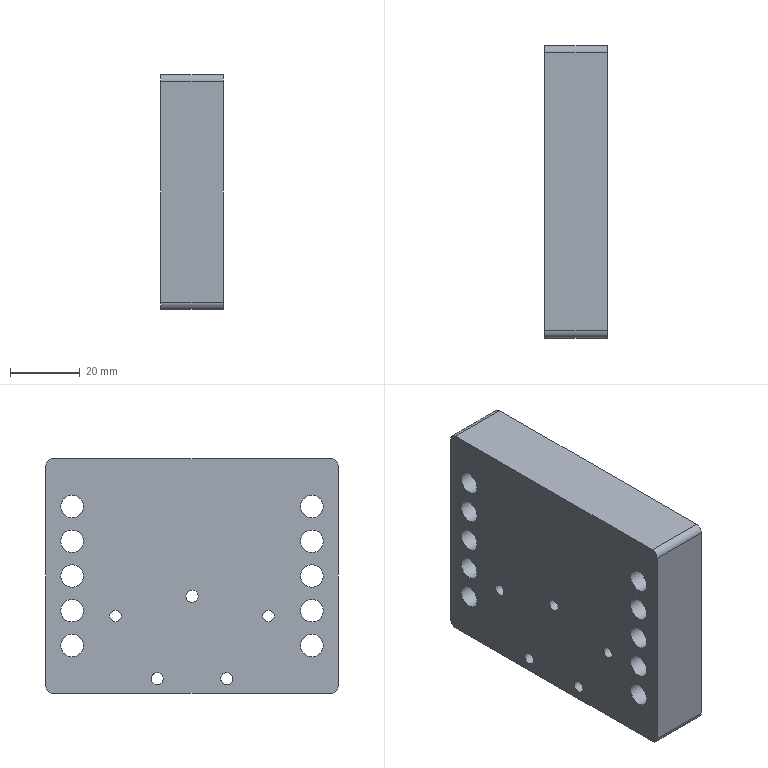Part | NX | 1 solid | 31 faces | box 18 x 84 x 67.5 mm | volume 94862 mm3 | cylinder 22 | plane 9 | commonest cylinder face diameters 6.5 x10 4 x4 3.5 x3 6 x3 3.3 x2
STEP:
#1=CARTESIAN_POINT('',(-224.,-62.153,788.95));
#2=VERTEX_POINT('',#1);
#3=CARTESIAN_POINT('',(-224.,-65.403,788.95));
#4=DIRECTION('',(1.,0.,0.));
#5=DIRECTION('',(0.,1.,0.));
#6=AXIS2_PLACEMENT_3D('',#3,#4,#5);
#7=CIRCLE('',#6,3.25);
#8=EDGE_CURVE('',#2,#2,#7,.T.);
#9=ORIENTED_EDGE('',*,*,#8,.T.);
#10=EDGE_LOOP('',(#9));
#11=FACE_BOUND('',#10,.T.);
#12=CARTESIAN_POINT('',(-224.,-62.153,778.95));
#13=VERTEX_POINT('',#12);
#14=CARTESIAN_POINT('',(-224.,-65.403,778.95));
#15=DIRECTION('',(1.,0.,0.));
#16=DIRECTION('',(0.,1.,0.));
#17=AXIS2_PLACEMENT_3D('',#14,#15,#16);
#18=CIRCLE('',#17,3.25);
#19=EDGE_CURVE('',#13,#13,#18,.T.);
#20=ORIENTED_EDGE('',*,*,#19,.T.);
#21=EDGE_LOOP('',(#20));
#22=FACE_BOUND('',#21,.T.);
#23=CARTESIAN_POINT('',(-224.,-62.153,748.95));
#24=VERTEX_POINT('',#23);
#25=CARTESIAN_POINT('',(-224.,-65.403,748.95));
#26=DIRECTION('',(1.,0.,0.));
#27=DIRECTION('',(0.,1.,0.));
#28=AXIS2_PLACEMENT_3D('',#25,#26,#27);
#29=CIRCLE('',#28,3.25);
#30=EDGE_CURVE('',#24,#24,#29,.T.);
#31=ORIENTED_EDGE('',*,*,#30,.T.);
#32=EDGE_LOOP('',(#31));
#33=FACE_BOUND('',#32,.T.);
#34=CARTESIAN_POINT('',(-224.,-62.153,758.95));
#35=VERTEX_POINT('',#34);
#36=CARTESIAN_POINT('',(-224.,-65.403,758.95));
#37=DIRECTION('',(1.,0.,0.));
#38=DIRECTION('',(0.,1.,0.));
#39=AXIS2_PLACEMENT_3D('',#36,#37,#38);
#40=CIRCLE('',#39,3.25);
#41=EDGE_CURVE('',#35,#35,#40,.T.);
#42=ORIENTED_EDGE('',*,*,#41,.T.);
#43=EDGE_LOOP('',(#42));
#44=FACE_BOUND('',#43,.T.);
#45=CARTESIAN_POINT('',(-224.,-62.153,768.95));
#46=VERTEX_POINT('',#45);
#47=CARTESIAN_POINT('',(-224.,-65.403,768.95));
#48=DIRECTION('',(1.,0.,0.));
#49=DIRECTION('',(0.,1.,0.));
#50=AXIS2_PLACEMENT_3D('',#47,#48,#49);
#51=CIRCLE('',#50,3.25);
#52=EDGE_CURVE('',#46,#46,#51,.T.);
#53=ORIENTED_EDGE('',*,*,#52,.T.);
#54=EDGE_LOOP('',(#53));
#55=FACE_BOUND('',#54,.T.);
#56=CARTESIAN_POINT('',(-224.,-131.153,748.95));
#57=VERTEX_POINT('',#56);
#58=CARTESIAN_POINT('',(-224.,-134.403,748.95));
#59=DIRECTION('',(1.,0.,0.));
#60=DIRECTION('',(0.,1.,0.));
#61=AXIS2_PLACEMENT_3D('',#58,#59,#60);
#62=CIRCLE('',#61,3.25);
#63=EDGE_CURVE('',#57,#57,#62,.T.);
#64=ORIENTED_EDGE('',*,*,#63,.T.);
#65=EDGE_LOOP('',(#64));
#66=FACE_BOUND('',#65,.T.);
#67=CARTESIAN_POINT('',(-224.,-131.153,758.95));
#68=VERTEX_POINT('',#67);
#69=CARTESIAN_POINT('',(-224.,-134.403,758.95));
#70=DIRECTION('',(1.,0.,0.));
#71=DIRECTION('',(0.,1.,0.));
#72=AXIS2_PLACEMENT_3D('',#69,#70,#71);
#73=CIRCLE('',#72,3.25);
#74=EDGE_CURVE('',#68,#68,#73,.T.);
#75=ORIENTED_EDGE('',*,*,#74,.T.);
#76=EDGE_LOOP('',(#75));
#77=FACE_BOUND('',#76,.T.);
#78=CARTESIAN_POINT('',(-224.,-131.153,788.95));
#79=VERTEX_POINT('',#78);
#80=CARTESIAN_POINT('',(-224.,-134.403,788.95));
#81=DIRECTION('',(1.,0.,0.));
#82=DIRECTION('',(0.,1.,0.));
#83=AXIS2_PLACEMENT_3D('',#80,#81,#82);
#84=CIRCLE('',#83,3.25);
#85=EDGE_CURVE('',#79,#79,#84,.T.);
#86=ORIENTED_EDGE('',*,*,#85,.T.);
#87=EDGE_LOOP('',(#86));
#88=FACE_BOUND('',#87,.T.);
#89=CARTESIAN_POINT('',(-224.,-131.153,778.95));
#90=VERTEX_POINT('',#89);
#91=CARTESIAN_POINT('',(-224.,-134.403,778.95));
#92=DIRECTION('',(1.,0.,0.));
#93=DIRECTION('',(0.,1.,0.));
#94=AXIS2_PLACEMENT_3D('',#91,#92,#93);
#95=CIRCLE('',#94,3.25);
#96=EDGE_CURVE('',#90,#90,#95,.T.);
#97=ORIENTED_EDGE('',*,*,#96,.T.);
#98=EDGE_LOOP('',(#97));
#99=FACE_BOUND('',#98,.T.);
#100=CARTESIAN_POINT('',(-224.,-131.153,768.95));
#101=VERTEX_POINT('',#100);
#102=CARTESIAN_POINT('',(-224.,-134.403,768.95));
#103=DIRECTION('',(1.,0.,0.));
#104=DIRECTION('',(0.,1.,0.));
#105=AXIS2_PLACEMENT_3D('',#102,#103,#104);
#106=CIRCLE('',#105,3.25);
#107=EDGE_CURVE('',#101,#101,#106,.T.);
#108=ORIENTED_EDGE('',*,*,#107,.T.);
#109=EDGE_LOOP('',(#108));
#110=FACE_BOUND('',#109,.T.);
#111=CARTESIAN_POINT('',(-224.,-120.253,757.45));
#112=VERTEX_POINT('',#111);
#113=CARTESIAN_POINT('',(-224.,-121.903,757.45));
#114=DIRECTION('',(-1.,0.,0.));
#115=DIRECTION('',(0.,1.,0.));
#116=AXIS2_PLACEMENT_3D('',#113,#114,#115);
#117=CIRCLE('',#116,1.65);
#118=EDGE_CURVE('',#112,#112,#117,.T.);
#119=ORIENTED_EDGE('',*,*,#118,.F.);
#120=EDGE_LOOP('',(#119));
#121=FACE_BOUND('',#120,.T.);
#122=CARTESIAN_POINT('',(-224.,-76.253,757.45));
#123=VERTEX_POINT('',#122);
#124=CARTESIAN_POINT('',(-224.,-77.903,757.45));
#125=DIRECTION('',(-1.,0.,0.));
#126=DIRECTION('',(0.,1.,0.));
#127=AXIS2_PLACEMENT_3D('',#124,#125,#126);
#128=CIRCLE('',#127,1.65);
#129=EDGE_CURVE('',#123,#123,#128,.T.);
#130=ORIENTED_EDGE('',*,*,#129,.F.);
#131=EDGE_LOOP('',(#130));
#132=FACE_BOUND('',#131,.T.);
#133=CARTESIAN_POINT('',(-224.,-108.153,739.4));
#134=VERTEX_POINT('',#133);
#135=CARTESIAN_POINT('',(-224.,-109.903,739.4));
#136=DIRECTION('',(1.,0.,0.));
#137=DIRECTION('',(0.,1.,0.));
#138=AXIS2_PLACEMENT_3D('',#135,#136,#137);
#139=CIRCLE('',#138,1.75);
#140=EDGE_CURVE('',#134,#134,#139,.T.);
#141=ORIENTED_EDGE('',*,*,#140,.T.);
#142=EDGE_LOOP('',(#141));
#143=FACE_BOUND('',#142,.T.);
#144=CARTESIAN_POINT('',(-224.,-88.153,739.4));
#145=VERTEX_POINT('',#144);
#146=CARTESIAN_POINT('',(-224.,-89.903,739.4));
#147=DIRECTION('',(1.,0.,0.));
#148=DIRECTION('',(0.,1.,0.));
#149=AXIS2_PLACEMENT_3D('',#146,#147,#148);
#150=CIRCLE('',#149,1.75);
#151=EDGE_CURVE('',#145,#145,#150,.T.);
#152=ORIENTED_EDGE('',*,*,#151,.T.);
#153=EDGE_LOOP('',(#152));
#154=FACE_BOUND('',#153,.T.);
#155=CARTESIAN_POINT('',(-224.,-98.153,763.1));
#156=VERTEX_POINT('',#155);
#157=CARTESIAN_POINT('',(-224.,-99.903,763.1));
#158=DIRECTION('',(1.,0.,0.));
#159=DIRECTION('',(0.,1.,0.));
#160=AXIS2_PLACEMENT_3D('',#157,#158,#159);
#161=CIRCLE('',#160,1.75);
#162=EDGE_CURVE('',#156,#156,#161,.T.);
#163=ORIENTED_EDGE('',*,*,#162,.T.);
#164=EDGE_LOOP('',(#163));
#165=FACE_BOUND('',#164,.T.);
#166=CARTESIAN_POINT('',(-224.,-139.903,735.2));
#167=VERTEX_POINT('',#166);
#168=CARTESIAN_POINT('',(-224.,-59.903,735.2));
#169=VERTEX_POINT('',#168);
#170=CARTESIAN_POINT('',(-224.,-75.403,735.2));
#171=DIRECTION('',(0.,1.,0.));
#172=VECTOR('',#171,1000.);
#173=LINE('',#170,#172);
#174=EDGE_CURVE('',#167,#169,#173,.T.);
#175=ORIENTED_EDGE('',*,*,#174,.F.);
#176=CARTESIAN_POINT('',(-224.,-141.903,737.2));
#177=VERTEX_POINT('',#176);
#178=CARTESIAN_POINT('',(-224.,-139.903,737.2));
#179=DIRECTION('',(1.,0.,0.));
#180=DIRECTION('',(0.,1.,0.));
#181=AXIS2_PLACEMENT_3D('',#178,#179,#180);
#182=CIRCLE('',#181,2.);
#183=EDGE_CURVE('',#167,#177,#182,.F.);
#184=ORIENTED_EDGE('',*,*,#183,.T.);
#185=CARTESIAN_POINT('',(-224.,-141.903,800.7));
#186=VERTEX_POINT('',#185);
#187=CARTESIAN_POINT('',(-224.,-141.903,736.2));
#188=DIRECTION('',(0.,0.,1.));
#189=VECTOR('',#188,1000.);
#190=LINE('',#187,#189);
#191=EDGE_CURVE('',#177,#186,#190,.T.);
#192=ORIENTED_EDGE('',*,*,#191,.T.);
#193=CARTESIAN_POINT('',(-224.,-139.903,802.7));
#194=VERTEX_POINT('',#193);
#195=CARTESIAN_POINT('',(-224.,-139.903,800.7));
#196=DIRECTION('',(1.,0.,0.));
#197=DIRECTION('',(0.,1.,0.));
#198=AXIS2_PLACEMENT_3D('',#195,#196,#197);
#199=CIRCLE('',#198,2.);
#200=EDGE_CURVE('',#186,#194,#199,.F.);
#201=ORIENTED_EDGE('',*,*,#200,.T.);
#202=CARTESIAN_POINT('',(-224.,-59.903,802.7));
#203=VERTEX_POINT('',#202);
#204=CARTESIAN_POINT('',(-224.,-102.903,802.7));
#205=DIRECTION('',(0.,1.,0.));
#206=VECTOR('',#205,1000.);
#207=LINE('',#204,#206);
#208=EDGE_CURVE('',#194,#203,#207,.T.);
#209=ORIENTED_EDGE('',*,*,#208,.T.);
#210=CARTESIAN_POINT('',(-224.,-57.903,800.7));
#211=VERTEX_POINT('',#210);
#212=CARTESIAN_POINT('',(-224.,-59.903,800.7));
#213=DIRECTION('',(1.,0.,0.));
#214=DIRECTION('',(0.,1.,0.));
#215=AXIS2_PLACEMENT_3D('',#212,#213,#214);
#216=CIRCLE('',#215,2.);
#217=EDGE_CURVE('',#203,#211,#216,.F.);
#218=ORIENTED_EDGE('',*,*,#217,.T.);
#219=CARTESIAN_POINT('',(-224.,-57.903,737.2));
#220=VERTEX_POINT('',#219);
#221=CARTESIAN_POINT('',(-224.,-57.903,269.15));
#222=DIRECTION('',(0.,0.,-1.));
#223=VECTOR('',#222,1000.);
#224=LINE('',#221,#223);
#225=EDGE_CURVE('',#211,#220,#224,.T.);
#226=ORIENTED_EDGE('',*,*,#225,.T.);
#227=CARTESIAN_POINT('',(-224.,-59.903,737.2));
#228=DIRECTION('',(1.,0.,0.));
#229=DIRECTION('',(0.,1.,0.));
#230=AXIS2_PLACEMENT_3D('',#227,#228,#229);
#231=CIRCLE('',#230,2.);
#232=EDGE_CURVE('',#220,#169,#231,.F.);
#233=ORIENTED_EDGE('',*,*,#232,.T.);
#234=EDGE_LOOP('',(#175,#184,#192,#201,#209,#218,#226,#233));
#235=FACE_BOUND('',#234,.T.);
#236=CARTESIAN_POINT('',(-224.,-95.403,757.2));
#237=DIRECTION('',(1.,0.,0.));
#238=DIRECTION('',(0.,0.,1.));
#239=AXIS2_PLACEMENT_3D('',#236,#237,#238);
#240=PLANE('',#239);
#241=ADVANCED_FACE('',(#11,#22,#33,#44,#55,#66,#77,#88,#99,#110,#121,#132,#143,#154,#165,#235),#240,.F.);
#242=ORIENTED_EDGE('',*,*,#8,.F.);
#243=EDGE_LOOP('',(#242));
#244=FACE_BOUND('',#243,.T.);
#245=CARTESIAN_POINT('',(-206.,-62.153,788.95));
#246=VERTEX_POINT('',#245);
#247=CARTESIAN_POINT('',(-206.,-65.403,788.95));
#248=DIRECTION('',(1.,0.,0.));
#249=DIRECTION('',(0.,1.,0.));
#250=AXIS2_PLACEMENT_3D('',#247,#248,#249);
#251=CIRCLE('',#250,3.25);
#252=EDGE_CURVE('',#246,#246,#251,.T.);
#253=ORIENTED_EDGE('',*,*,#252,.T.);
#254=EDGE_LOOP('',(#253));
#255=FACE_BOUND('',#254,.T.);
#256=CARTESIAN_POINT('',(-196.,-65.403,788.95));
#257=DIRECTION('',(-1.,0.,0.));
#258=DIRECTION('',(0.,0.,-1.));
#259=AXIS2_PLACEMENT_3D('',#256,#257,#258);
#260=CYLINDRICAL_SURFACE('',#259,3.25);
#261=ADVANCED_FACE('',(#244,#255),#260,.F.);
#262=ORIENTED_EDGE('',*,*,#19,.F.);
#263=EDGE_LOOP('',(#262));
#264=FACE_BOUND('',#263,.T.);
#265=CARTESIAN_POINT('',(-206.,-62.153,778.95));
#266=VERTEX_POINT('',#265);
#267=CARTESIAN_POINT('',(-206.,-65.403,778.95));
#268=DIRECTION('',(1.,0.,0.));
#269=DIRECTION('',(0.,1.,0.));
#270=AXIS2_PLACEMENT_3D('',#267,#268,#269);
#271=CIRCLE('',#270,3.25);
#272=EDGE_CURVE('',#266,#266,#271,.T.);
#273=ORIENTED_EDGE('',*,*,#272,.T.);
#274=EDGE_LOOP('',(#273));
#275=FACE_BOUND('',#274,.T.);
#276=CARTESIAN_POINT('',(-196.,-65.403,778.95));
#277=DIRECTION('',(-1.,0.,0.));
#278=DIRECTION('',(0.,0.,-1.));
#279=AXIS2_PLACEMENT_3D('',#276,#277,#278);
#280=CYLINDRICAL_SURFACE('',#279,3.25);
#281=ADVANCED_FACE('',(#264,#275),#280,.F.);
#282=ORIENTED_EDGE('',*,*,#30,.F.);
#283=EDGE_LOOP('',(#282));
#284=FACE_BOUND('',#283,.T.);
#285=CARTESIAN_POINT('',(-206.,-62.153,748.95));
#286=VERTEX_POINT('',#285);
#287=CARTESIAN_POINT('',(-206.,-65.403,748.95));
#288=DIRECTION('',(1.,0.,0.));
#289=DIRECTION('',(0.,1.,0.));
#290=AXIS2_PLACEMENT_3D('',#287,#288,#289);
#291=CIRCLE('',#290,3.25);
#292=EDGE_CURVE('',#286,#286,#291,.T.);
#293=ORIENTED_EDGE('',*,*,#292,.T.);
#294=EDGE_LOOP('',(#293));
#295=FACE_BOUND('',#294,.T.);
#296=CARTESIAN_POINT('',(-196.,-65.403,748.95));
#297=DIRECTION('',(-1.,0.,0.));
#298=DIRECTION('',(0.,0.,-1.));
#299=AXIS2_PLACEMENT_3D('',#296,#297,#298);
#300=CYLINDRICAL_SURFACE('',#299,3.25);
#301=ADVANCED_FACE('',(#284,#295),#300,.F.);
#302=ORIENTED_EDGE('',*,*,#41,.F.);
#303=EDGE_LOOP('',(#302));
#304=FACE_BOUND('',#303,.T.);
#305=CARTESIAN_POINT('',(-206.,-62.153,758.95));
#306=VERTEX_POINT('',#305);
#307=CARTESIAN_POINT('',(-206.,-65.403,758.95));
#308=DIRECTION('',(1.,0.,0.));
#309=DIRECTION('',(0.,1.,0.));
#310=AXIS2_PLACEMENT_3D('',#307,#308,#309);
#311=CIRCLE('',#310,3.25);
#312=EDGE_CURVE('',#306,#306,#311,.T.);
#313=ORIENTED_EDGE('',*,*,#312,.T.);
#314=EDGE_LOOP('',(#313));
#315=FACE_BOUND('',#314,.T.);
#316=CARTESIAN_POINT('',(-196.,-65.403,758.95));
#317=DIRECTION('',(-1.,0.,0.));
#318=DIRECTION('',(0.,0.,-1.));
#319=AXIS2_PLACEMENT_3D('',#316,#317,#318);
#320=CYLINDRICAL_SURFACE('',#319,3.25);
#321=ADVANCED_FACE('',(#304,#315),#320,.F.);
#322=ORIENTED_EDGE('',*,*,#52,.F.);
#323=EDGE_LOOP('',(#322));
#324=FACE_BOUND('',#323,.T.);
#325=CARTESIAN_POINT('',(-206.,-62.153,768.95));
#326=VERTEX_POINT('',#325);
#327=CARTESIAN_POINT('',(-206.,-65.403,768.95));
#328=DIRECTION('',(1.,0.,0.));
#329=DIRECTION('',(0.,1.,0.));
#330=AXIS2_PLACEMENT_3D('',#327,#328,#329);
#331=CIRCLE('',#330,3.25);
#332=EDGE_CURVE('',#326,#326,#331,.T.);
#333=ORIENTED_EDGE('',*,*,#332,.T.);
#334=EDGE_LOOP('',(#333));
#335=FACE_BOUND('',#334,.T.);
#336=CARTESIAN_POINT('',(-196.,-65.403,768.95));
#337=DIRECTION('',(-1.,0.,0.));
#338=DIRECTION('',(0.,0.,-1.));
#339=AXIS2_PLACEMENT_3D('',#336,#337,#338);
#340=CYLINDRICAL_SURFACE('',#339,3.25);
#341=ADVANCED_FACE('',(#324,#335),#340,.F.);
#342=ORIENTED_EDGE('',*,*,#63,.F.);
#343=EDGE_LOOP('',(#342));
#344=FACE_BOUND('',#343,.T.);
#345=CARTESIAN_POINT('',(-206.,-131.153,748.95));
#346=VERTEX_POINT('',#345);
#347=CARTESIAN_POINT('',(-206.,-134.403,748.95));
#348=DIRECTION('',(1.,0.,0.));
#349=DIRECTION('',(0.,1.,0.));
#350=AXIS2_PLACEMENT_3D('',#347,#348,#349);
#351=CIRCLE('',#350,3.25);
#352=EDGE_CURVE('',#346,#346,#351,.T.);
#353=ORIENTED_EDGE('',*,*,#352,.T.);
#354=EDGE_LOOP('',(#353));
#355=FACE_BOUND('',#354,.T.);
#356=CARTESIAN_POINT('',(-196.,-134.403,748.95));
#357=DIRECTION('',(-1.,0.,0.));
#358=DIRECTION('',(0.,0.,-1.));
#359=AXIS2_PLACEMENT_3D('',#356,#357,#358);
#360=CYLINDRICAL_SURFACE('',#359,3.25);
#361=ADVANCED_FACE('',(#344,#355),#360,.F.);
#362=ORIENTED_EDGE('',*,*,#74,.F.);
#363=EDGE_LOOP('',(#362));
#364=FACE_BOUND('',#363,.T.);
#365=CARTESIAN_POINT('',(-206.,-131.153,758.95));
#366=VERTEX_POINT('',#365);
#367=CARTESIAN_POINT('',(-206.,-134.403,758.95));
#368=DIRECTION('',(1.,0.,0.));
#369=DIRECTION('',(0.,1.,0.));
#370=AXIS2_PLACEMENT_3D('',#367,#368,#369);
#371=CIRCLE('',#370,3.25);
#372=EDGE_CURVE('',#366,#366,#371,.T.);
#373=ORIENTED_EDGE('',*,*,#372,.T.);
#374=EDGE_LOOP('',(#373));
#375=FACE_BOUND('',#374,.T.);
#376=CARTESIAN_POINT('',(-196.,-134.403,758.95));
#377=DIRECTION('',(-1.,0.,0.));
#378=DIRECTION('',(0.,0.,-1.));
#379=AXIS2_PLACEMENT_3D('',#376,#377,#378);
#380=CYLINDRICAL_SURFACE('',#379,3.25);
#381=ADVANCED_FACE('',(#364,#375),#380,.F.);
#382=ORIENTED_EDGE('',*,*,#85,.F.);
#383=EDGE_LOOP('',(#382));
#384=FACE_BOUND('',#383,.T.);
#385=CARTESIAN_POINT('',(-206.,-131.153,788.95));
#386=VERTEX_POINT('',#385);
#387=CARTESIAN_POINT('',(-206.,-134.403,788.95));
#388=DIRECTION('',(1.,0.,0.));
#389=DIRECTION('',(0.,1.,0.));
#390=AXIS2_PLACEMENT_3D('',#387,#388,#389);
#391=CIRCLE('',#390,3.25);
#392=EDGE_CURVE('',#386,#386,#391,.T.);
#393=ORIENTED_EDGE('',*,*,#392,.T.);
#394=EDGE_LOOP('',(#393));
#395=FACE_BOUND('',#394,.T.);
#396=CARTESIAN_POINT('',(-196.,-134.403,788.95));
#397=DIRECTION('',(-1.,0.,0.));
#398=DIRECTION('',(0.,0.,-1.));
#399=AXIS2_PLACEMENT_3D('',#396,#397,#398);
#400=CYLINDRICAL_SURFACE('',#399,3.25);
#401=ADVANCED_FACE('',(#384,#395),#400,.F.);
#402=ORIENTED_EDGE('',*,*,#96,.F.);
#403=EDGE_LOOP('',(#402));
#404=FACE_BOUND('',#403,.T.);
#405=CARTESIAN_POINT('',(-206.,-131.153,778.95));
#406=VERTEX_POINT('',#405);
#407=CARTESIAN_POINT('',(-206.,-134.403,778.95));
#408=DIRECTION('',(1.,0.,0.));
#409=DIRECTION('',(0.,1.,0.));
#410=AXIS2_PLACEMENT_3D('',#407,#408,#409);
#411=CIRCLE('',#410,3.25);
#412=EDGE_CURVE('',#406,#406,#411,.T.);
#413=ORIENTED_EDGE('',*,*,#412,.T.);
#414=EDGE_LOOP('',(#413));
#415=FACE_BOUND('',#414,.T.);
#416=CARTESIAN_POINT('',(-196.,-134.403,778.95));
#417=DIRECTION('',(-1.,0.,0.));
#418=DIRECTION('',(0.,0.,-1.));
#419=AXIS2_PLACEMENT_3D('',#416,#417,#418);
#420=CYLINDRICAL_SURFACE('',#419,3.25);
#421=ADVANCED_FACE('',(#404,#415),#420,.F.);
#422=ORIENTED_EDGE('',*,*,#107,.F.);
#423=EDGE_LOOP('',(#422));
#424=FACE_BOUND('',#423,.T.);
#425=CARTESIAN_POINT('',(-206.,-131.153,768.95));
#426=VERTEX_POINT('',#425);
#427=CARTESIAN_POINT('',(-206.,-134.403,768.95));
#428=DIRECTION('',(1.,0.,0.));
#429=DIRECTION('',(0.,1.,0.));
#430=AXIS2_PLACEMENT_3D('',#427,#428,#429);
#431=CIRCLE('',#430,3.25);
#432=EDGE_CURVE('',#426,#426,#431,.T.);
#433=ORIENTED_EDGE('',*,*,#432,.T.);
#434=EDGE_LOOP('',(#433));
#435=FACE_BOUND('',#434,.T.);
#436=CARTESIAN_POINT('',(-196.,-134.403,768.95));
#437=DIRECTION('',(-1.,0.,0.));
#438=DIRECTION('',(0.,0.,-1.));
#439=AXIS2_PLACEMENT_3D('',#436,#437,#438);
#440=CYLINDRICAL_SURFACE('',#439,3.25);
#441=ADVANCED_FACE('',(#424,#435),#440,.F.);
#442=CARTESIAN_POINT('',(-212.,-99.903,764.85));
#443=VERTEX_POINT('',#442);
#444=CARTESIAN_POINT('',(-212.,-99.903,763.1));
#445=DIRECTION('',(1.,0.,0.));
#446=DIRECTION('',(0.,0.,1.));
#447=AXIS2_PLACEMENT_3D('',#444,#445,#446);
#448=CIRCLE('',#447,1.75);
#449=EDGE_CURVE('',#443,#443,#448,.T.);
#450=ORIENTED_EDGE('',*,*,#449,.F.);
#451=EDGE_LOOP('',(#450));
#452=FACE_BOUND('',#451,.T.);
#453=CARTESIAN_POINT('',(-212.,-99.903,766.1));
#454=VERTEX_POINT('',#453);
#455=CARTESIAN_POINT('',(-212.,-99.903,763.1));
#456=DIRECTION('',(-1.,0.,0.));
#457=DIRECTION('',(0.,0.,1.));
#458=AXIS2_PLACEMENT_3D('',#455,#456,#457);
#459=CIRCLE('',#458,3.);
#460=EDGE_CURVE('',#454,#454,#459,.T.);
#461=ORIENTED_EDGE('',*,*,#460,.F.);
#462=EDGE_LOOP('',(#461));
#463=FACE_BOUND('',#462,.T.);
#464=CARTESIAN_POINT('',(-212.,-99.903,768.95));
#465=DIRECTION('',(-1.,0.,0.));
#466=DIRECTION('',(0.,0.,1.));
#467=AXIS2_PLACEMENT_3D('',#464,#465,#466);
#468=PLANE('',#467);
#469=ADVANCED_FACE('',(#452,#463),#468,.F.);
#470=ORIENTED_EDGE('',*,*,#140,.F.);
#471=EDGE_LOOP('',(#470));
#472=FACE_BOUND('',#471,.T.);
#473=CARTESIAN_POINT('',(-212.,-109.903,741.15));
#474=VERTEX_POINT('',#473);
#475=CARTESIAN_POINT('',(-212.,-109.903,739.4));
#476=DIRECTION('',(-1.,0.,0.));
#477=DIRECTION('',(0.,0.,1.));
#478=AXIS2_PLACEMENT_3D('',#475,#476,#477);
#479=CIRCLE('',#478,1.75);
#480=EDGE_CURVE('',#474,#474,#479,.T.);
#481=ORIENTED_EDGE('',*,*,#480,.F.);
#482=EDGE_LOOP('',(#481));
#483=FACE_BOUND('',#482,.T.);
#484=CARTESIAN_POINT('',(-214.,-109.903,739.4));
#485=DIRECTION('',(1.,0.,0.));
#486=DIRECTION('',(0.,0.,1.));
#487=AXIS2_PLACEMENT_3D('',#484,#485,#486);
#488=CYLINDRICAL_SURFACE('',#487,1.75);
#489=ADVANCED_FACE('',(#472,#483),#488,.F.);
#490=ORIENTED_EDGE('',*,*,#151,.F.);
#491=EDGE_LOOP('',(#490));
#492=FACE_BOUND('',#491,.T.);
#493=CARTESIAN_POINT('',(-212.,-89.903,741.15));
#494=VERTEX_POINT('',#493);
#495=CARTESIAN_POINT('',(-212.,-89.903,739.4));
#496=DIRECTION('',(-1.,0.,0.));
#497=DIRECTION('',(0.,0.,1.));
#498=AXIS2_PLACEMENT_3D('',#495,#496,#497);
#499=CIRCLE('',#498,1.75);
#500=EDGE_CURVE('',#494,#494,#499,.T.);
#501=ORIENTED_EDGE('',*,*,#500,.F.);
#502=EDGE_LOOP('',(#501));
#503=FACE_BOUND('',#502,.T.);
#504=CARTESIAN_POINT('',(-214.,-89.903,739.4));
#505=DIRECTION('',(1.,0.,0.));
#506=DIRECTION('',(0.,0.,1.));
#507=AXIS2_PLACEMENT_3D('',#504,#505,#506);
#508=CYLINDRICAL_SURFACE('',#507,1.75);
#509=ADVANCED_FACE('',(#492,#503),#508,.F.);
#510=ORIENTED_EDGE('',*,*,#162,.F.);
#511=EDGE_LOOP('',(#510));
#512=FACE_BOUND('',#511,.T.);
#513=ORIENTED_EDGE('',*,*,#449,.T.);
#514=EDGE_LOOP('',(#513));
#515=FACE_BOUND('',#514,.T.);
#516=CARTESIAN_POINT('',(-214.,-99.903,763.1));
#517=DIRECTION('',(1.,0.,0.));
#518=DIRECTION('',(0.,0.,1.));
#519=AXIS2_PLACEMENT_3D('',#516,#517,#518);
#520=CYLINDRICAL_SURFACE('',#519,1.75);
#521=ADVANCED_FACE('',(#512,#515),#520,.F.);
#522=CARTESIAN_POINT('',(-212.,-109.903,742.4));
#523=VERTEX_POINT('',#522);
#524=CARTESIAN_POINT('',(-212.,-109.903,739.4));
#525=DIRECTION('',(1.,0.,0.));
#526=DIRECTION('',(0.,0.,1.));
#527=AXIS2_PLACEMENT_3D('',#524,#525,#526);
#528=CIRCLE('',#527,3.);
#529=EDGE_CURVE('',#523,#523,#528,.T.);
#530=ORIENTED_EDGE('',*,*,#529,.T.);
#531=EDGE_LOOP('',(#530));
#532=FACE_BOUND('',#531,.T.);
#533=ORIENTED_EDGE('',*,*,#480,.T.);
#534=EDGE_LOOP('',(#533));
#535=FACE_BOUND('',#534,.T.);
#536=CARTESIAN_POINT('',(-212.,-99.903,768.95));
#537=DIRECTION('',(-1.,0.,0.));
#538=DIRECTION('',(0.,0.,1.));
#539=AXIS2_PLACEMENT_3D('',#536,#537,#538);
#540=PLANE('',#539);
#541=ADVANCED_FACE('',(#532,#535),#540,.F.);
#542=CARTESIAN_POINT('',(-212.,-89.903,742.4));
#543=VERTEX_POINT('',#542);
#544=CARTESIAN_POINT('',(-212.,-89.903,739.4));
#545=DIRECTION('',(1.,0.,0.));
#546=DIRECTION('',(0.,0.,1.));
#547=AXIS2_PLACEMENT_3D('',#544,#545,#546);
#548=CIRCLE('',#547,3.);
#549=EDGE_CURVE('',#543,#543,#548,.T.);
#550=ORIENTED_EDGE('',*,*,#549,.T.);
#551=EDGE_LOOP('',(#550));
#552=FACE_BOUND('',#551,.T.);
#553=ORIENTED_EDGE('',*,*,#500,.T.);
#554=EDGE_LOOP('',(#553));
#555=FACE_BOUND('',#554,.T.);
#556=CARTESIAN_POINT('',(-212.,-99.903,768.95));
#557=DIRECTION('',(-1.,0.,0.));
#558=DIRECTION('',(0.,0.,1.));
#559=AXIS2_PLACEMENT_3D('',#556,#557,#558);
#560=PLANE('',#559);
#561=ADVANCED_FACE('',(#552,#555),#560,.F.);
#562=ORIENTED_EDGE('',*,*,#183,.F.);
#563=CARTESIAN_POINT('',(-206.,-139.903,735.2));
#564=VERTEX_POINT('',#563);
#565=CARTESIAN_POINT('',(-224.,-139.903,735.2));
#566=DIRECTION('',(-1.,0.,0.));
#567=VECTOR('',#566,1000.);
#568=LINE('',#565,#567);
#569=EDGE_CURVE('',#564,#167,#568,.T.);
#570=ORIENTED_EDGE('',*,*,#569,.F.);
#571=CARTESIAN_POINT('',(-206.,-141.903,737.2));
#572=VERTEX_POINT('',#571);
#573=CARTESIAN_POINT('',(-206.,-139.903,737.2));
#574=DIRECTION('',(1.,0.,0.));
#575=DIRECTION('',(0.,1.,0.));
#576=AXIS2_PLACEMENT_3D('',#573,#574,#575);
#577=CIRCLE('',#576,2.);
#578=EDGE_CURVE('',#572,#564,#577,.T.);
#579=ORIENTED_EDGE('',*,*,#578,.F.);
#580=CARTESIAN_POINT('',(-204.,-141.903,737.2));
#581=DIRECTION('',(1.,0.,0.));
#582=VECTOR('',#581,1000.);
#583=LINE('',#580,#582);
#584=EDGE_CURVE('',#177,#572,#583,.T.);
#585=ORIENTED_EDGE('',*,*,#584,.F.);
#586=EDGE_LOOP('',(#562,#570,#579,#585));
#587=FACE_BOUND('',#586,.T.);
#588=CARTESIAN_POINT('',(-224.,-139.903,737.2));
#589=DIRECTION('',(1.,0.,0.));
#590=DIRECTION('',(0.,0.,-1.));
#591=AXIS2_PLACEMENT_3D('',#588,#589,#590);
#592=CYLINDRICAL_SURFACE('',#591,2.);
#593=ADVANCED_FACE('',(#587),#592,.T.);
#594=ORIENTED_EDGE('',*,*,#200,.F.);
#595=CARTESIAN_POINT('',(-206.,-141.903,800.7));
#596=VERTEX_POINT('',#595);
#597=CARTESIAN_POINT('',(-204.,-141.903,800.7));
#598=DIRECTION('',(-1.,0.,0.));
#599=VECTOR('',#598,1000.);
#600=LINE('',#597,#599);
#601=EDGE_CURVE('',#596,#186,#600,.T.);
#602=ORIENTED_EDGE('',*,*,#601,.F.);
#603=CARTESIAN_POINT('',(-206.,-139.903,802.7));
#604=VERTEX_POINT('',#603);
#605=CARTESIAN_POINT('',(-206.,-139.903,800.7));
#606=DIRECTION('',(1.,0.,0.));
#607=DIRECTION('',(0.,1.,0.));
#608=AXIS2_PLACEMENT_3D('',#605,#606,#607);
#609=CIRCLE('',#608,2.);
#610=EDGE_CURVE('',#604,#596,#609,.T.);
#611=ORIENTED_EDGE('',*,*,#610,.F.);
#612=CARTESIAN_POINT('',(-204.,-139.903,802.7));
#613=DIRECTION('',(1.,0.,0.));
#614=VECTOR('',#613,1000.);
#615=LINE('',#612,#614);
#616=EDGE_CURVE('',#194,#604,#615,.T.);
#617=ORIENTED_EDGE('',*,*,#616,.F.);
#618=EDGE_LOOP('',(#594,#602,#611,#617));
#619=FACE_BOUND('',#618,.T.);
#620=CARTESIAN_POINT('',(-204.,-139.903,800.7));
#621=DIRECTION('',(1.,0.,0.));
#622=DIRECTION('',(0.,0.,-1.));
#623=AXIS2_PLACEMENT_3D('',#620,#621,#622);
#624=CYLINDRICAL_SURFACE('',#623,2.);
#625=ADVANCED_FACE('',(#619),#624,.T.);
#626=ORIENTED_EDGE('',*,*,#217,.F.);
#627=CARTESIAN_POINT('',(-206.,-59.903,802.7));
#628=VERTEX_POINT('',#627);
#629=CARTESIAN_POINT('',(-204.,-59.903,802.7));
#630=DIRECTION('',(-1.,0.,0.));
#631=VECTOR('',#630,1000.);
#632=LINE('',#629,#631);
#633=EDGE_CURVE('',#628,#203,#632,.T.);
#634=ORIENTED_EDGE('',*,*,#633,.F.);
#635=CARTESIAN_POINT('',(-206.,-57.903,800.7));
#636=VERTEX_POINT('',#635);
#637=CARTESIAN_POINT('',(-206.,-59.903,800.7));
#638=DIRECTION('',(1.,0.,0.));
#639=DIRECTION('',(0.,1.,0.));
#640=AXIS2_PLACEMENT_3D('',#637,#638,#639);
#641=CIRCLE('',#640,2.);
#642=EDGE_CURVE('',#636,#628,#641,.T.);
#643=ORIENTED_EDGE('',*,*,#642,.F.);
#644=CARTESIAN_POINT('',(-42.25,-57.903,800.7));
#645=DIRECTION('',(1.,0.,0.));
#646=VECTOR('',#645,1000.);
#647=LINE('',#644,#646);
#648=EDGE_CURVE('',#211,#636,#647,.T.);
#649=ORIENTED_EDGE('',*,*,#648,.F.);
#650=EDGE_LOOP('',(#626,#634,#643,#649));
#651=FACE_BOUND('',#650,.T.);
#652=CARTESIAN_POINT('',(-42.25,-59.903,800.7));
#653=DIRECTION('',(1.,0.,0.));
#654=DIRECTION('',(0.,0.,-1.));
#655=AXIS2_PLACEMENT_3D('',#652,#653,#654);
#656=CYLINDRICAL_SURFACE('',#655,2.);
#657=ADVANCED_FACE('',(#651),#656,.T.);
#658=ORIENTED_EDGE('',*,*,#232,.F.);
#659=CARTESIAN_POINT('',(-206.,-57.903,737.2));
#660=VERTEX_POINT('',#659);
#661=CARTESIAN_POINT('',(-42.25,-57.903,737.2));
#662=DIRECTION('',(-1.,0.,0.));
#663=VECTOR('',#662,1000.);
#664=LINE('',#661,#663);
#665=EDGE_CURVE('',#660,#220,#664,.T.);
#666=ORIENTED_EDGE('',*,*,#665,.F.);
#667=CARTESIAN_POINT('',(-206.,-59.903,735.2));
#668=VERTEX_POINT('',#667);
#669=CARTESIAN_POINT('',(-206.,-59.903,737.2));
#670=DIRECTION('',(1.,0.,0.));
#671=DIRECTION('',(0.,1.,0.));
#672=AXIS2_PLACEMENT_3D('',#669,#670,#671);
#673=CIRCLE('',#672,2.);
#674=EDGE_CURVE('',#668,#660,#673,.T.);
#675=ORIENTED_EDGE('',*,*,#674,.F.);
#676=CARTESIAN_POINT('',(-224.,-59.903,735.2));
#677=DIRECTION('',(1.,0.,0.));
#678=VECTOR('',#677,1000.);
#679=LINE('',#676,#678);
#680=EDGE_CURVE('',#169,#668,#679,.T.);
#681=ORIENTED_EDGE('',*,*,#680,.F.);
#682=EDGE_LOOP('',(#658,#666,#675,#681));
#683=FACE_BOUND('',#682,.T.);
#684=CARTESIAN_POINT('',(-42.25,-59.903,737.2));
#685=DIRECTION('',(1.,0.,0.));
#686=DIRECTION('',(0.,0.,-1.));
#687=AXIS2_PLACEMENT_3D('',#684,#685,#686);
#688=CYLINDRICAL_SURFACE('',#687,2.);
#689=ADVANCED_FACE('',(#683),#688,.T.);
#690=ORIENTED_EDGE('',*,*,#191,.F.);
#691=ORIENTED_EDGE('',*,*,#584,.T.);
#692=CARTESIAN_POINT('',(-206.,-141.903,757.2));
#693=DIRECTION('',(0.,0.,1.));
#694=VECTOR('',#693,1000.);
#695=LINE('',#692,#694);
#696=EDGE_CURVE('',#572,#596,#695,.T.);
#697=ORIENTED_EDGE('',*,*,#696,.T.);
#698=ORIENTED_EDGE('',*,*,#601,.T.);
#699=EDGE_LOOP('',(#690,#691,#697,#698));
#700=FACE_BOUND('',#699,.T.);
#701=CARTESIAN_POINT('',(-204.,-141.903,736.2));
#702=DIRECTION('',(0.,-1.,0.));
#703=DIRECTION('',(0.,0.,-1.));
#704=AXIS2_PLACEMENT_3D('',#701,#702,#703);
#705=PLANE('',#704);
#706=ADVANCED_FACE('',(#700),#705,.T.);
#707=ORIENTED_EDGE('',*,*,#225,.F.);
#708=ORIENTED_EDGE('',*,*,#648,.T.);
#709=CARTESIAN_POINT('',(-206.,-57.903,269.15));
#710=DIRECTION('',(0.,0.,1.));
#711=VECTOR('',#710,1000.);
#712=LINE('',#709,#711);
#713=EDGE_CURVE('',#660,#636,#712,.T.);
#714=ORIENTED_EDGE('',*,*,#713,.F.);
#715=ORIENTED_EDGE('',*,*,#665,.T.);
#716=EDGE_LOOP('',(#707,#708,#714,#715));
#717=FACE_BOUND('',#716,.T.);
#718=CARTESIAN_POINT('',(-42.25,-57.903,269.15));
#719=DIRECTION('',(0.,1.,0.));
#720=DIRECTION('',(0.,0.,1.));
#721=AXIS2_PLACEMENT_3D('',#718,#719,#720);
#722=PLANE('',#721);
#723=ADVANCED_FACE('',(#717),#722,.T.);
#724=CARTESIAN_POINT('',(-206.,-99.903,735.2));
#725=DIRECTION('',(0.,-1.,0.));
#726=VECTOR('',#725,1000.);
#727=LINE('',#724,#726);
#728=EDGE_CURVE('',#668,#564,#727,.T.);
#729=ORIENTED_EDGE('',*,*,#728,.F.);
#730=ORIENTED_EDGE('',*,*,#674,.T.);
#731=ORIENTED_EDGE('',*,*,#713,.T.);
#732=ORIENTED_EDGE('',*,*,#642,.T.);
#733=CARTESIAN_POINT('',(-206.,-102.903,802.7));
#734=DIRECTION('',(0.,-1.,0.));
#735=VECTOR('',#734,1000.);
#736=LINE('',#733,#735);
#737=EDGE_CURVE('',#628,#604,#736,.T.);
#738=ORIENTED_EDGE('',*,*,#737,.T.);
#739=ORIENTED_EDGE('',*,*,#610,.T.);
#740=ORIENTED_EDGE('',*,*,#696,.F.);
#741=ORIENTED_EDGE('',*,*,#578,.T.);
#742=EDGE_LOOP('',(#729,#730,#731,#732,#738,#739,#740,#741));
#743=FACE_BOUND('',#742,.T.);
#744=CARTESIAN_POINT('',(-206.,-96.903,763.1));
#745=VERTEX_POINT('',#744);
#746=CARTESIAN_POINT('',(-206.,-99.903,763.1));
#747=DIRECTION('',(1.,0.,0.));
#748=DIRECTION('',(0.,1.,0.));
#749=AXIS2_PLACEMENT_3D('',#746,#747,#748);
#750=CIRCLE('',#749,3.);
#751=EDGE_CURVE('',#745,#745,#750,.T.);
#752=ORIENTED_EDGE('',*,*,#751,.F.);
#753=EDGE_LOOP('',(#752));
#754=FACE_BOUND('',#753,.T.);
#755=CARTESIAN_POINT('',(-206.,-106.903,739.4));
#756=VERTEX_POINT('',#755);
#757=CARTESIAN_POINT('',(-206.,-109.903,739.4));
#758=DIRECTION('',(1.,0.,0.));
#759=DIRECTION('',(0.,1.,0.));
#760=AXIS2_PLACEMENT_3D('',#757,#758,#759);
#761=CIRCLE('',#760,3.);
#762=EDGE_CURVE('',#756,#756,#761,.T.);
#763=ORIENTED_EDGE('',*,*,#762,.F.);
#764=EDGE_LOOP('',(#763));
#765=FACE_BOUND('',#764,.T.);
#766=CARTESIAN_POINT('',(-206.,-86.903,739.4));
#767=VERTEX_POINT('',#766);
#768=CARTESIAN_POINT('',(-206.,-89.903,739.4));
#769=DIRECTION('',(-1.,0.,0.));
#770=DIRECTION('',(0.,1.,0.));
#771=AXIS2_PLACEMENT_3D('',#768,#769,#770);
#772=CIRCLE('',#771,3.);
#773=EDGE_CURVE('',#767,#767,#772,.T.);
#774=ORIENTED_EDGE('',*,*,#773,.T.);
#775=EDGE_LOOP('',(#774));
#776=FACE_BOUND('',#775,.T.);
#777=CARTESIAN_POINT('',(-206.,-76.253,757.45));
#778=VERTEX_POINT('',#777);
#779=CARTESIAN_POINT('',(-206.,-77.903,757.45));
#780=DIRECTION('',(-1.,0.,0.));
#781=DIRECTION('',(0.,1.,0.));
#782=AXIS2_PLACEMENT_3D('',#779,#780,#781);
#783=CIRCLE('',#782,1.65);
#784=EDGE_CURVE('',#778,#778,#783,.T.);
#785=ORIENTED_EDGE('',*,*,#784,.T.);
#786=EDGE_LOOP('',(#785));
#787=FACE_BOUND('',#786,.T.);
#788=CARTESIAN_POINT('',(-206.,-120.253,757.45));
#789=VERTEX_POINT('',#788);
#790=CARTESIAN_POINT('',(-206.,-121.903,757.45));
#791=DIRECTION('',(-1.,0.,0.));
#792=DIRECTION('',(0.,1.,0.));
#793=AXIS2_PLACEMENT_3D('',#790,#791,#792);
#794=CIRCLE('',#793,1.65);
#795=EDGE_CURVE('',#789,#789,#794,.T.);
#796=ORIENTED_EDGE('',*,*,#795,.T.);
#797=EDGE_LOOP('',(#796));
#798=FACE_BOUND('',#797,.T.);
#799=ORIENTED_EDGE('',*,*,#432,.F.);
#800=EDGE_LOOP('',(#799));
#801=FACE_BOUND('',#800,.T.);
#802=ORIENTED_EDGE('',*,*,#412,.F.);
#803=EDGE_LOOP('',(#802));
#804=FACE_BOUND('',#803,.T.);
#805=ORIENTED_EDGE('',*,*,#392,.F.);
#806=EDGE_LOOP('',(#805));
#807=FACE_BOUND('',#806,.T.);
#808=ORIENTED_EDGE('',*,*,#372,.F.);
#809=EDGE_LOOP('',(#808));
#810=FACE_BOUND('',#809,.T.);
#811=ORIENTED_EDGE('',*,*,#352,.F.);
#812=EDGE_LOOP('',(#811));
#813=FACE_BOUND('',#812,.T.);
#814=ORIENTED_EDGE('',*,*,#332,.F.);
#815=EDGE_LOOP('',(#814));
#816=FACE_BOUND('',#815,.T.);
#817=ORIENTED_EDGE('',*,*,#312,.F.);
#818=EDGE_LOOP('',(#817));
#819=FACE_BOUND('',#818,.T.);
#820=ORIENTED_EDGE('',*,*,#292,.F.);
#821=EDGE_LOOP('',(#820));
#822=FACE_BOUND('',#821,.T.);
#823=ORIENTED_EDGE('',*,*,#272,.F.);
#824=EDGE_LOOP('',(#823));
#825=FACE_BOUND('',#824,.T.);
#826=ORIENTED_EDGE('',*,*,#252,.F.);
#827=EDGE_LOOP('',(#826));
#828=FACE_BOUND('',#827,.T.);
#829=CARTESIAN_POINT('',(-206.,-99.903,757.2));
#830=DIRECTION('',(1.,0.,0.));
#831=DIRECTION('',(0.,1.,0.));
#832=AXIS2_PLACEMENT_3D('',#829,#830,#831);
#833=PLANE('',#832);
#834=ADVANCED_FACE('',(#743,#754,#765,#776,#787,#798,#801,#804,#807,#810,#813,#816,#819,#822,#825,#828),#833,.T.);
#835=ORIENTED_EDGE('',*,*,#118,.T.);
#836=EDGE_LOOP('',(#835));
#837=FACE_BOUND('',#836,.T.);
#838=ORIENTED_EDGE('',*,*,#795,.F.);
#839=EDGE_LOOP('',(#838));
#840=FACE_BOUND('',#839,.T.);
#841=CARTESIAN_POINT('',(-259.,-121.903,757.45));
#842=DIRECTION('',(1.,0.,0.));
#843=DIRECTION('',(0.,0.,-1.));
#844=AXIS2_PLACEMENT_3D('',#841,#842,#843);
#845=CYLINDRICAL_SURFACE('',#844,1.65);
#846=ADVANCED_FACE('',(#837,#840),#845,.F.);
#847=ORIENTED_EDGE('',*,*,#129,.T.);
#848=EDGE_LOOP('',(#847));
#849=FACE_BOUND('',#848,.T.);
#850=ORIENTED_EDGE('',*,*,#784,.F.);
#851=EDGE_LOOP('',(#850));
#852=FACE_BOUND('',#851,.T.);
#853=CARTESIAN_POINT('',(-259.,-77.903,757.45));
#854=DIRECTION('',(1.,0.,0.));
#855=DIRECTION('',(0.,0.,-1.));
#856=AXIS2_PLACEMENT_3D('',#853,#854,#855);
#857=CYLINDRICAL_SURFACE('',#856,1.65);
#858=ADVANCED_FACE('',(#849,#852),#857,.F.);
#859=ORIENTED_EDGE('',*,*,#529,.F.);
#860=EDGE_LOOP('',(#859));
#861=FACE_BOUND('',#860,.T.);
#862=ORIENTED_EDGE('',*,*,#762,.T.);
#863=EDGE_LOOP('',(#862));
#864=FACE_BOUND('',#863,.T.);
#865=CARTESIAN_POINT('',(-214.,-109.903,739.4));
#866=DIRECTION('',(1.,0.,0.));
#867=DIRECTION('',(0.,0.,1.));
#868=AXIS2_PLACEMENT_3D('',#865,#866,#867);
#869=CYLINDRICAL_SURFACE('',#868,3.);
#870=ADVANCED_FACE('',(#861,#864),#869,.F.);
#871=ORIENTED_EDGE('',*,*,#549,.F.);
#872=EDGE_LOOP('',(#871));
#873=FACE_BOUND('',#872,.T.);
#874=ORIENTED_EDGE('',*,*,#773,.F.);
#875=EDGE_LOOP('',(#874));
#876=FACE_BOUND('',#875,.T.);
#877=CARTESIAN_POINT('',(-214.,-89.903,739.4));
#878=DIRECTION('',(1.,0.,0.));
#879=DIRECTION('',(0.,0.,1.));
#880=AXIS2_PLACEMENT_3D('',#877,#878,#879);
#881=CYLINDRICAL_SURFACE('',#880,3.);
#882=ADVANCED_FACE('',(#873,#876),#881,.F.);
#883=ORIENTED_EDGE('',*,*,#460,.T.);
#884=EDGE_LOOP('',(#883));
#885=FACE_BOUND('',#884,.T.);
#886=ORIENTED_EDGE('',*,*,#751,.T.);
#887=EDGE_LOOP('',(#886));
#888=FACE_BOUND('',#887,.T.);
#889=CARTESIAN_POINT('',(-214.,-99.903,763.1));
#890=DIRECTION('',(1.,0.,0.));
#891=DIRECTION('',(0.,0.,1.));
#892=AXIS2_PLACEMENT_3D('',#889,#890,#891);
#893=CYLINDRICAL_SURFACE('',#892,3.);
#894=ADVANCED_FACE('',(#885,#888),#893,.F.);
#895=ORIENTED_EDGE('',*,*,#208,.F.);
#896=ORIENTED_EDGE('',*,*,#616,.T.);
#897=ORIENTED_EDGE('',*,*,#737,.F.);
#898=ORIENTED_EDGE('',*,*,#633,.T.);
#899=EDGE_LOOP('',(#895,#896,#897,#898));
#900=FACE_BOUND('',#899,.T.);
#901=CARTESIAN_POINT('',(-204.,-102.903,802.7));
#902=DIRECTION('',(0.,0.,1.));
#903=DIRECTION('',(0.,-1.,0.));
#904=AXIS2_PLACEMENT_3D('',#901,#902,#903);
#905=PLANE('',#904);
#906=ADVANCED_FACE('',(#900),#905,.T.);
#907=ORIENTED_EDGE('',*,*,#569,.T.);
#908=ORIENTED_EDGE('',*,*,#174,.T.);
#909=ORIENTED_EDGE('',*,*,#680,.T.);
#910=ORIENTED_EDGE('',*,*,#728,.T.);
#911=EDGE_LOOP('',(#907,#908,#909,#910));
#912=FACE_BOUND('',#911,.T.);
#913=CARTESIAN_POINT('',(-224.,-75.403,735.2));
#914=DIRECTION('',(0.,0.,1.));
#915=DIRECTION('',(-1.,0.,0.));
#916=AXIS2_PLACEMENT_3D('',#913,#914,#915);
#917=PLANE('',#916);
#918=ADVANCED_FACE('',(#912),#917,.F.);
#919=CLOSED_SHELL('',(#241,#261,#281,#301,#321,#341,#361,#381,#401,#421,#441,#469,#489,#509,#521,#541,#561,#593,#625,#657,#689,#706,#723,#834,#846,#858,#870,#882,#894,#906,#918));
#920=MANIFOLD_SOLID_BREP('',#919);
#921=(LENGTH_UNIT()NAMED_UNIT(*)SI_UNIT(.MILLI.,.METRE.));
#922=UNCERTAINTY_MEASURE_WITH_UNIT(LENGTH_MEASURE(0.00001),#921,'','');
#923=(NAMED_UNIT(*)PLANE_ANGLE_UNIT()SI_UNIT($,.RADIAN.));
#924=(NAMED_UNIT(*)SI_UNIT($,.STERADIAN.)SOLID_ANGLE_UNIT());
#925=(GEOMETRIC_REPRESENTATION_CONTEXT(3)GLOBAL_UNCERTAINTY_ASSIGNED_CONTEXT((#922))GLOBAL_UNIT_ASSIGNED_CONTEXT((#921,#923,#924))REPRESENTATION_CONTEXT('',''));
#926=ADVANCED_BREP_SHAPE_REPRESENTATION('',(#920),#925);